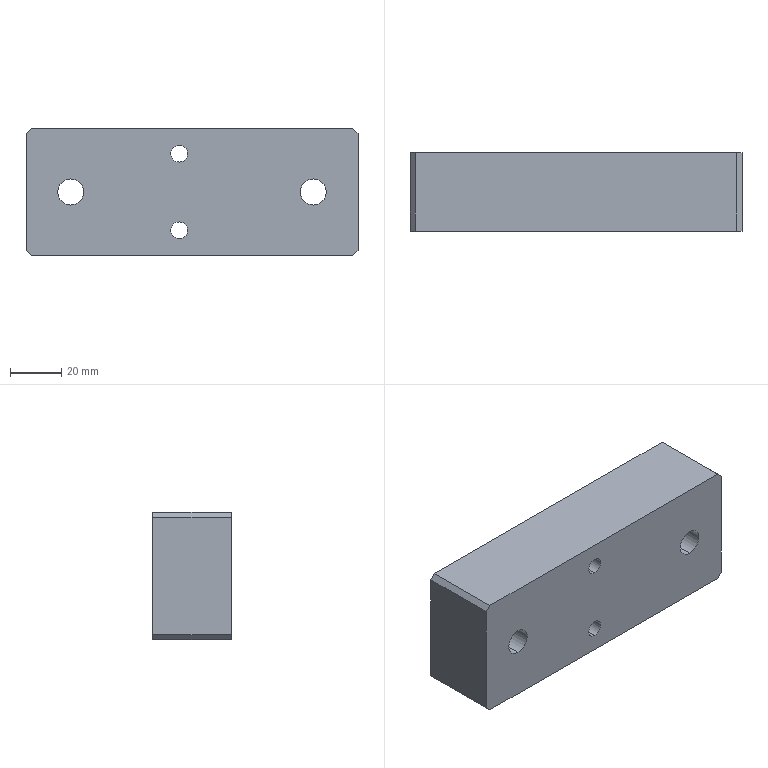Part | SolidWorks | features HoleWzd 2, Chamfer 1, Extrusion 1 | 1 solid | 24 faces | box 130 x 30.7 x 50 mm | volume 191359 mm3 | cylinder 12 | plane 12 | commonest cylinder face diameters 6.6 x4 10.2 x4 11 x4
STEP:
#1=CARTESIAN_POINT('',(-5.,8.55,9.5));
#2=VERTEX_POINT('',#1);
#3=CARTESIAN_POINT('',(-5.,8.55,20.5));
#4=VERTEX_POINT('',#3);
#5=CARTESIAN_POINT('',(-5.,8.55,15.));
#6=DIRECTION('',(0.,1.,0.));
#7=DIRECTION('',(0.,0.,1.));
#8=AXIS2_PLACEMENT_3D('',#5,#6,#7);
#9=CIRCLE('',#8,5.5);
#10=EDGE_CURVE('',#2,#4,#9,.T.);
#11=ORIENTED_EDGE('',*,*,#10,.F.);
#12=CARTESIAN_POINT('',(-5.,15.35,9.5));
#13=VERTEX_POINT('',#12);
#14=CARTESIAN_POINT('',(-5.,15.35,9.5));
#15=DIRECTION('',(0.,1.,0.));
#16=VECTOR('',#15,1000.);
#17=LINE('',#14,#16);
#18=EDGE_CURVE('',#2,#13,#17,.T.);
#19=ORIENTED_EDGE('',*,*,#18,.T.);
#20=CARTESIAN_POINT('',(-5.,15.35,20.5));
#21=VERTEX_POINT('',#20);
#22=CARTESIAN_POINT('',(-5.,15.35,15.));
#23=DIRECTION('',(0.,1.,0.));
#24=DIRECTION('',(0.,0.,1.));
#25=AXIS2_PLACEMENT_3D('',#22,#23,#24);
#26=CIRCLE('',#25,5.5);
#27=EDGE_CURVE('',#13,#21,#26,.T.);
#28=ORIENTED_EDGE('',*,*,#27,.T.);
#29=CARTESIAN_POINT('',(-5.,15.35,20.5));
#30=DIRECTION('',(0.,1.,0.));
#31=VECTOR('',#30,1000.);
#32=LINE('',#29,#31);
#33=EDGE_CURVE('',#4,#21,#32,.T.);
#34=ORIENTED_EDGE('',*,*,#33,.F.);
#35=EDGE_LOOP('',(#11,#19,#28,#34));
#36=FACE_OUTER_BOUND('',#35,.T.);
#37=CARTESIAN_POINT('',(-5.,15.35,15.));
#38=DIRECTION('',(0.,1.,0.));
#39=DIRECTION('',(0.,0.,1.));
#40=AXIS2_PLACEMENT_3D('',#37,#38,#39);
#41=CYLINDRICAL_SURFACE('',#40,5.5);
#42=ADVANCED_FACE('',(#36),#41,.F.);
#43=CARTESIAN_POINT('',(-5.,-15.35,11.7));
#44=VERTEX_POINT('',#43);
#45=CARTESIAN_POINT('',(-5.,-15.35,18.3));
#46=VERTEX_POINT('',#45);
#47=CARTESIAN_POINT('',(-5.,-15.35,15.));
#48=DIRECTION('',(0.,1.,0.));
#49=DIRECTION('',(0.,0.,1.));
#50=AXIS2_PLACEMENT_3D('',#47,#48,#49);
#51=CIRCLE('',#50,3.3);
#52=EDGE_CURVE('',#44,#46,#51,.T.);
#53=ORIENTED_EDGE('',*,*,#52,.F.);
#54=CARTESIAN_POINT('',(-5.,8.55,11.7));
#55=VERTEX_POINT('',#54);
#56=CARTESIAN_POINT('',(-5.,15.35,11.7));
#57=DIRECTION('',(0.,1.,0.));
#58=VECTOR('',#57,1000.);
#59=LINE('',#56,#58);
#60=EDGE_CURVE('',#44,#55,#59,.T.);
#61=ORIENTED_EDGE('',*,*,#60,.T.);
#62=CARTESIAN_POINT('',(-5.,8.55,18.3));
#63=VERTEX_POINT('',#62);
#64=CARTESIAN_POINT('',(-5.,8.55,15.));
#65=DIRECTION('',(0.,1.,0.));
#66=DIRECTION('',(0.,0.,1.));
#67=AXIS2_PLACEMENT_3D('',#64,#65,#66);
#68=CIRCLE('',#67,3.3);
#69=EDGE_CURVE('',#55,#63,#68,.T.);
#70=ORIENTED_EDGE('',*,*,#69,.T.);
#71=CARTESIAN_POINT('',(-5.,15.35,18.3));
#72=DIRECTION('',(0.,1.,0.));
#73=VECTOR('',#72,1000.);
#74=LINE('',#71,#73);
#75=EDGE_CURVE('',#46,#63,#74,.T.);
#76=ORIENTED_EDGE('',*,*,#75,.F.);
#77=EDGE_LOOP('',(#53,#61,#70,#76));
#78=FACE_OUTER_BOUND('',#77,.T.);
#79=CARTESIAN_POINT('',(-5.,15.35,15.));
#80=DIRECTION('',(0.,1.,0.));
#81=DIRECTION('',(0.,0.,1.));
#82=AXIS2_PLACEMENT_3D('',#79,#80,#81);
#83=CYLINDRICAL_SURFACE('',#82,3.3);
#84=ADVANCED_FACE('',(#78),#83,.F.);
#85=CARTESIAN_POINT('',(-5.,8.55,-20.5));
#86=VERTEX_POINT('',#85);
#87=CARTESIAN_POINT('',(-5.,8.55,-9.5));
#88=VERTEX_POINT('',#87);
#89=CARTESIAN_POINT('',(-5.,8.55,-15.));
#90=DIRECTION('',(0.,1.,0.));
#91=DIRECTION('',(0.,0.,1.));
#92=AXIS2_PLACEMENT_3D('',#89,#90,#91);
#93=CIRCLE('',#92,5.5);
#94=EDGE_CURVE('',#86,#88,#93,.T.);
#95=ORIENTED_EDGE('',*,*,#94,.F.);
#96=CARTESIAN_POINT('',(-5.,15.35,-20.5));
#97=VERTEX_POINT('',#96);
#98=CARTESIAN_POINT('',(-5.,15.35,-20.5));
#99=DIRECTION('',(0.,1.,0.));
#100=VECTOR('',#99,1000.);
#101=LINE('',#98,#100);
#102=EDGE_CURVE('',#86,#97,#101,.T.);
#103=ORIENTED_EDGE('',*,*,#102,.T.);
#104=CARTESIAN_POINT('',(-5.,15.35,-9.5));
#105=VERTEX_POINT('',#104);
#106=CARTESIAN_POINT('',(-5.,15.35,-15.));
#107=DIRECTION('',(0.,1.,0.));
#108=DIRECTION('',(0.,0.,1.));
#109=AXIS2_PLACEMENT_3D('',#106,#107,#108);
#110=CIRCLE('',#109,5.5);
#111=EDGE_CURVE('',#97,#105,#110,.T.);
#112=ORIENTED_EDGE('',*,*,#111,.T.);
#113=CARTESIAN_POINT('',(-5.,15.35,-9.5));
#114=DIRECTION('',(0.,1.,0.));
#115=VECTOR('',#114,1000.);
#116=LINE('',#113,#115);
#117=EDGE_CURVE('',#88,#105,#116,.T.);
#118=ORIENTED_EDGE('',*,*,#117,.F.);
#119=EDGE_LOOP('',(#95,#103,#112,#118));
#120=FACE_OUTER_BOUND('',#119,.T.);
#121=CARTESIAN_POINT('',(-5.,15.35,-15.));
#122=DIRECTION('',(0.,1.,0.));
#123=DIRECTION('',(0.,0.,1.));
#124=AXIS2_PLACEMENT_3D('',#121,#122,#123);
#125=CYLINDRICAL_SURFACE('',#124,5.5);
#126=ADVANCED_FACE('',(#120),#125,.F.);
#127=CARTESIAN_POINT('',(-5.,-15.35,-18.3));
#128=VERTEX_POINT('',#127);
#129=CARTESIAN_POINT('',(-5.,-15.35,-11.7));
#130=VERTEX_POINT('',#129);
#131=CARTESIAN_POINT('',(-5.,-15.35,-15.));
#132=DIRECTION('',(0.,1.,0.));
#133=DIRECTION('',(0.,0.,1.));
#134=AXIS2_PLACEMENT_3D('',#131,#132,#133);
#135=CIRCLE('',#134,3.3);
#136=EDGE_CURVE('',#128,#130,#135,.T.);
#137=ORIENTED_EDGE('',*,*,#136,.F.);
#138=CARTESIAN_POINT('',(-5.,8.55,-18.3));
#139=VERTEX_POINT('',#138);
#140=CARTESIAN_POINT('',(-5.,15.35,-18.3));
#141=DIRECTION('',(0.,1.,0.));
#142=VECTOR('',#141,1000.);
#143=LINE('',#140,#142);
#144=EDGE_CURVE('',#128,#139,#143,.T.);
#145=ORIENTED_EDGE('',*,*,#144,.T.);
#146=CARTESIAN_POINT('',(-5.,8.55,-11.7));
#147=VERTEX_POINT('',#146);
#148=CARTESIAN_POINT('',(-5.,8.55,-15.));
#149=DIRECTION('',(0.,1.,0.));
#150=DIRECTION('',(0.,0.,1.));
#151=AXIS2_PLACEMENT_3D('',#148,#149,#150);
#152=CIRCLE('',#151,3.3);
#153=EDGE_CURVE('',#139,#147,#152,.T.);
#154=ORIENTED_EDGE('',*,*,#153,.T.);
#155=CARTESIAN_POINT('',(-5.,15.35,-11.7));
#156=DIRECTION('',(0.,1.,0.));
#157=VECTOR('',#156,1000.);
#158=LINE('',#155,#157);
#159=EDGE_CURVE('',#130,#147,#158,.T.);
#160=ORIENTED_EDGE('',*,*,#159,.F.);
#161=EDGE_LOOP('',(#137,#145,#154,#160));
#162=FACE_OUTER_BOUND('',#161,.T.);
#163=CARTESIAN_POINT('',(-5.,15.35,-15.));
#164=DIRECTION('',(0.,1.,0.));
#165=DIRECTION('',(0.,0.,1.));
#166=AXIS2_PLACEMENT_3D('',#163,#164,#165);
#167=CYLINDRICAL_SURFACE('',#166,3.3);
#168=ADVANCED_FACE('',(#162),#167,.F.);
#169=CARTESIAN_POINT('',(-47.5,-15.35,-5.1));
#170=VERTEX_POINT('',#169);
#171=CARTESIAN_POINT('',(-47.5,-15.35,5.1));
#172=VERTEX_POINT('',#171);
#173=CARTESIAN_POINT('',(-47.5,-15.35,0.));
#174=DIRECTION('',(0.,1.,0.));
#175=DIRECTION('',(0.,0.,1.));
#176=AXIS2_PLACEMENT_3D('',#173,#174,#175);
#177=CIRCLE('',#176,5.1);
#178=EDGE_CURVE('',#170,#172,#177,.T.);
#179=ORIENTED_EDGE('',*,*,#178,.F.);
#180=CARTESIAN_POINT('',(-47.5,15.35,-5.1));
#181=VERTEX_POINT('',#180);
#182=CARTESIAN_POINT('',(-47.5,15.35,-5.1));
#183=DIRECTION('',(0.,1.,0.));
#184=VECTOR('',#183,1000.);
#185=LINE('',#182,#184);
#186=EDGE_CURVE('',#170,#181,#185,.T.);
#187=ORIENTED_EDGE('',*,*,#186,.T.);
#188=CARTESIAN_POINT('',(-47.5,15.35,5.1));
#189=VERTEX_POINT('',#188);
#190=CARTESIAN_POINT('',(-47.5,15.35,0.));
#191=DIRECTION('',(0.,1.,0.));
#192=DIRECTION('',(0.,0.,1.));
#193=AXIS2_PLACEMENT_3D('',#190,#191,#192);
#194=CIRCLE('',#193,5.1);
#195=EDGE_CURVE('',#181,#189,#194,.T.);
#196=ORIENTED_EDGE('',*,*,#195,.T.);
#197=CARTESIAN_POINT('',(-47.5,15.35,5.1));
#198=DIRECTION('',(0.,1.,0.));
#199=VECTOR('',#198,1000.);
#200=LINE('',#197,#199);
#201=EDGE_CURVE('',#172,#189,#200,.T.);
#202=ORIENTED_EDGE('',*,*,#201,.F.);
#203=EDGE_LOOP('',(#179,#187,#196,#202));
#204=FACE_OUTER_BOUND('',#203,.T.);
#205=CARTESIAN_POINT('',(-47.5,15.35,0.));
#206=DIRECTION('',(0.,1.,0.));
#207=DIRECTION('',(0.,0.,1.));
#208=AXIS2_PLACEMENT_3D('',#205,#206,#207);
#209=CYLINDRICAL_SURFACE('',#208,5.1);
#210=ADVANCED_FACE('',(#204),#209,.F.);
#211=CARTESIAN_POINT('',(47.5,-15.35,-5.1));
#212=VERTEX_POINT('',#211);
#213=CARTESIAN_POINT('',(47.5,-15.35,5.1));
#214=VERTEX_POINT('',#213);
#215=CARTESIAN_POINT('',(47.5,-15.35,0.));
#216=DIRECTION('',(0.,1.,0.));
#217=DIRECTION('',(0.,0.,1.));
#218=AXIS2_PLACEMENT_3D('',#215,#216,#217);
#219=CIRCLE('',#218,5.1);
#220=EDGE_CURVE('',#212,#214,#219,.T.);
#221=ORIENTED_EDGE('',*,*,#220,.F.);
#222=CARTESIAN_POINT('',(47.5,15.35,-5.1));
#223=VERTEX_POINT('',#222);
#224=CARTESIAN_POINT('',(47.5,15.35,-5.1));
#225=DIRECTION('',(0.,1.,0.));
#226=VECTOR('',#225,1000.);
#227=LINE('',#224,#226);
#228=EDGE_CURVE('',#212,#223,#227,.T.);
#229=ORIENTED_EDGE('',*,*,#228,.T.);
#230=CARTESIAN_POINT('',(47.5,15.35,5.1));
#231=VERTEX_POINT('',#230);
#232=CARTESIAN_POINT('',(47.5,15.35,0.));
#233=DIRECTION('',(0.,1.,0.));
#234=DIRECTION('',(0.,0.,1.));
#235=AXIS2_PLACEMENT_3D('',#232,#233,#234);
#236=CIRCLE('',#235,5.1);
#237=EDGE_CURVE('',#223,#231,#236,.T.);
#238=ORIENTED_EDGE('',*,*,#237,.T.);
#239=CARTESIAN_POINT('',(47.5,15.35,5.1));
#240=DIRECTION('',(0.,1.,0.));
#241=VECTOR('',#240,1000.);
#242=LINE('',#239,#241);
#243=EDGE_CURVE('',#214,#231,#242,.T.);
#244=ORIENTED_EDGE('',*,*,#243,.F.);
#245=EDGE_LOOP('',(#221,#229,#238,#244));
#246=FACE_OUTER_BOUND('',#245,.T.);
#247=CARTESIAN_POINT('',(47.5,15.35,0.));
#248=DIRECTION('',(0.,1.,0.));
#249=DIRECTION('',(0.,0.,1.));
#250=AXIS2_PLACEMENT_3D('',#247,#248,#249);
#251=CYLINDRICAL_SURFACE('',#250,5.1);
#252=ADVANCED_FACE('',(#246),#251,.F.);
#253=CARTESIAN_POINT('',(65.,-15.35,23.));
#254=VERTEX_POINT('',#253);
#255=CARTESIAN_POINT('',(65.,-15.35,-23.));
#256=VERTEX_POINT('',#255);
#257=CARTESIAN_POINT('',(65.,-15.35,25.));
#258=DIRECTION('',(0.,0.,-1.));
#259=VECTOR('',#258,1000.);
#260=LINE('',#257,#259);
#261=EDGE_CURVE('',#254,#256,#260,.T.);
#262=ORIENTED_EDGE('',*,*,#261,.T.);
#263=CARTESIAN_POINT('',(65.,15.35,-23.));
#264=VERTEX_POINT('',#263);
#265=CARTESIAN_POINT('',(65.,15.35,-23.));
#266=DIRECTION('',(0.,1.,0.));
#267=VECTOR('',#266,1000.);
#268=LINE('',#265,#267);
#269=EDGE_CURVE('',#256,#264,#268,.T.);
#270=ORIENTED_EDGE('',*,*,#269,.T.);
#271=CARTESIAN_POINT('',(65.,15.35,23.));
#272=VERTEX_POINT('',#271);
#273=CARTESIAN_POINT('',(65.,15.35,25.));
#274=DIRECTION('',(0.,0.,-1.));
#275=VECTOR('',#274,1000.);
#276=LINE('',#273,#275);
#277=EDGE_CURVE('',#272,#264,#276,.T.);
#278=ORIENTED_EDGE('',*,*,#277,.F.);
#279=CARTESIAN_POINT('',(65.,15.35,23.));
#280=DIRECTION('',(0.,-1.,0.));
#281=VECTOR('',#280,1000.);
#282=LINE('',#279,#281);
#283=EDGE_CURVE('',#272,#254,#282,.T.);
#284=ORIENTED_EDGE('',*,*,#283,.T.);
#285=EDGE_LOOP('',(#262,#270,#278,#284));
#286=FACE_OUTER_BOUND('',#285,.T.);
#287=CARTESIAN_POINT('',(65.,15.35,25.));
#288=DIRECTION('',(-1.,0.,0.));
#289=DIRECTION('',(0.,0.,1.));
#290=AXIS2_PLACEMENT_3D('',#287,#288,#289);
#291=PLANE('',#290);
#292=ADVANCED_FACE('',(#286),#291,.F.);
#293=CARTESIAN_POINT('',(63.,15.35,-25.));
#294=VERTEX_POINT('',#293);
#295=CARTESIAN_POINT('',(-63.,15.35,-25.));
#296=VERTEX_POINT('',#295);
#297=CARTESIAN_POINT('',(-65.,15.35,-25.));
#298=DIRECTION('',(-1.,0.,0.));
#299=VECTOR('',#298,1000.);
#300=LINE('',#297,#299);
#301=EDGE_CURVE('',#294,#296,#300,.T.);
#302=ORIENTED_EDGE('',*,*,#301,.F.);
#303=CARTESIAN_POINT('',(63.,-15.35,-25.));
#304=VERTEX_POINT('',#303);
#305=CARTESIAN_POINT('',(63.,15.35,-25.));
#306=DIRECTION('',(0.,-1.,0.));
#307=VECTOR('',#306,1000.);
#308=LINE('',#305,#307);
#309=EDGE_CURVE('',#294,#304,#308,.T.);
#310=ORIENTED_EDGE('',*,*,#309,.T.);
#311=CARTESIAN_POINT('',(-63.,-15.35,-25.));
#312=VERTEX_POINT('',#311);
#313=CARTESIAN_POINT('',(-65.,-15.35,-25.));
#314=DIRECTION('',(-1.,0.,0.));
#315=VECTOR('',#314,1000.);
#316=LINE('',#313,#315);
#317=EDGE_CURVE('',#304,#312,#316,.T.);
#318=ORIENTED_EDGE('',*,*,#317,.T.);
#319=CARTESIAN_POINT('',(-63.,15.35,-25.));
#320=DIRECTION('',(0.,1.,0.));
#321=VECTOR('',#320,1000.);
#322=LINE('',#319,#321);
#323=EDGE_CURVE('',#312,#296,#322,.T.);
#324=ORIENTED_EDGE('',*,*,#323,.T.);
#325=EDGE_LOOP('',(#302,#310,#318,#324));
#326=FACE_OUTER_BOUND('',#325,.T.);
#327=CARTESIAN_POINT('',(-65.,15.35,-25.));
#328=DIRECTION('',(0.,0.,1.));
#329=DIRECTION('',(1.,0.,0.));
#330=AXIS2_PLACEMENT_3D('',#327,#328,#329);
#331=PLANE('',#330);
#332=ADVANCED_FACE('',(#326),#331,.F.);
#333=CARTESIAN_POINT('',(-65.,15.35,-23.));
#334=VERTEX_POINT('',#333);
#335=CARTESIAN_POINT('',(-65.,15.35,23.));
#336=VERTEX_POINT('',#335);
#337=CARTESIAN_POINT('',(-65.,15.35,25.));
#338=DIRECTION('',(0.,0.,1.));
#339=VECTOR('',#338,1000.);
#340=LINE('',#337,#339);
#341=EDGE_CURVE('',#334,#336,#340,.T.);
#342=ORIENTED_EDGE('',*,*,#341,.F.);
#343=CARTESIAN_POINT('',(-65.,-15.35,-23.));
#344=VERTEX_POINT('',#343);
#345=CARTESIAN_POINT('',(-65.,15.35,-23.));
#346=DIRECTION('',(0.,-1.,0.));
#347=VECTOR('',#346,1000.);
#348=LINE('',#345,#347);
#349=EDGE_CURVE('',#334,#344,#348,.T.);
#350=ORIENTED_EDGE('',*,*,#349,.T.);
#351=CARTESIAN_POINT('',(-65.,-15.35,23.));
#352=VERTEX_POINT('',#351);
#353=CARTESIAN_POINT('',(-65.,-15.35,25.));
#354=DIRECTION('',(0.,0.,1.));
#355=VECTOR('',#354,1000.);
#356=LINE('',#353,#355);
#357=EDGE_CURVE('',#344,#352,#356,.T.);
#358=ORIENTED_EDGE('',*,*,#357,.T.);
#359=CARTESIAN_POINT('',(-65.,15.35,23.));
#360=DIRECTION('',(0.,1.,0.));
#361=VECTOR('',#360,1000.);
#362=LINE('',#359,#361);
#363=EDGE_CURVE('',#352,#336,#362,.T.);
#364=ORIENTED_EDGE('',*,*,#363,.T.);
#365=EDGE_LOOP('',(#342,#350,#358,#364));
#366=FACE_OUTER_BOUND('',#365,.T.);
#367=CARTESIAN_POINT('',(-65.,15.35,25.));
#368=DIRECTION('',(1.,0.,0.));
#369=DIRECTION('',(0.,0.,-1.));
#370=AXIS2_PLACEMENT_3D('',#367,#368,#369);
#371=PLANE('',#370);
#372=ADVANCED_FACE('',(#366),#371,.F.);
#373=CARTESIAN_POINT('',(-63.,-15.35,25.));
#374=VERTEX_POINT('',#373);
#375=CARTESIAN_POINT('',(63.,-15.35,25.));
#376=VERTEX_POINT('',#375);
#377=CARTESIAN_POINT('',(-65.,-15.35,25.));
#378=DIRECTION('',(1.,0.,0.));
#379=VECTOR('',#378,1000.);
#380=LINE('',#377,#379);
#381=EDGE_CURVE('',#374,#376,#380,.T.);
#382=ORIENTED_EDGE('',*,*,#381,.T.);
#383=CARTESIAN_POINT('',(63.,15.35,25.));
#384=VERTEX_POINT('',#383);
#385=CARTESIAN_POINT('',(63.,15.35,25.));
#386=DIRECTION('',(0.,1.,0.));
#387=VECTOR('',#386,1000.);
#388=LINE('',#385,#387);
#389=EDGE_CURVE('',#376,#384,#388,.T.);
#390=ORIENTED_EDGE('',*,*,#389,.T.);
#391=CARTESIAN_POINT('',(-63.,15.35,25.));
#392=VERTEX_POINT('',#391);
#393=CARTESIAN_POINT('',(-65.,15.35,25.));
#394=DIRECTION('',(1.,0.,0.));
#395=VECTOR('',#394,1000.);
#396=LINE('',#393,#395);
#397=EDGE_CURVE('',#392,#384,#396,.T.);
#398=ORIENTED_EDGE('',*,*,#397,.F.);
#399=CARTESIAN_POINT('',(-63.,15.35,25.));
#400=DIRECTION('',(0.,-1.,0.));
#401=VECTOR('',#400,1000.);
#402=LINE('',#399,#401);
#403=EDGE_CURVE('',#392,#374,#402,.T.);
#404=ORIENTED_EDGE('',*,*,#403,.T.);
#405=EDGE_LOOP('',(#382,#390,#398,#404));
#406=FACE_OUTER_BOUND('',#405,.T.);
#407=CARTESIAN_POINT('',(-65.,15.35,25.));
#408=DIRECTION('',(0.,0.,-1.));
#409=DIRECTION('',(-1.,0.,0.));
#410=AXIS2_PLACEMENT_3D('',#407,#408,#409);
#411=PLANE('',#410);
#412=ADVANCED_FACE('',(#406),#411,.F.);
#413=CARTESIAN_POINT('',(-5.,15.35,15.));
#414=DIRECTION('',(0.,1.,0.));
#415=DIRECTION('',(0.,0.,1.));
#416=AXIS2_PLACEMENT_3D('',#413,#414,#415);
#417=CIRCLE('',#416,5.5);
#418=EDGE_CURVE('',#21,#13,#417,.T.);
#419=ORIENTED_EDGE('',*,*,#418,.F.);
#420=ORIENTED_EDGE('',*,*,#27,.F.);
#421=EDGE_LOOP('',(#419,#420));
#422=FACE_BOUND('',#421,.T.);
#423=CARTESIAN_POINT('',(-5.,15.35,-15.));
#424=DIRECTION('',(0.,1.,0.));
#425=DIRECTION('',(0.,0.,1.));
#426=AXIS2_PLACEMENT_3D('',#423,#424,#425);
#427=CIRCLE('',#426,5.5);
#428=EDGE_CURVE('',#105,#97,#427,.T.);
#429=ORIENTED_EDGE('',*,*,#428,.F.);
#430=ORIENTED_EDGE('',*,*,#111,.F.);
#431=EDGE_LOOP('',(#429,#430));
#432=FACE_BOUND('',#431,.T.);
#433=CARTESIAN_POINT('',(-47.5,15.35,0.));
#434=DIRECTION('',(0.,1.,0.));
#435=DIRECTION('',(0.,0.,1.));
#436=AXIS2_PLACEMENT_3D('',#433,#434,#435);
#437=CIRCLE('',#436,5.1);
#438=EDGE_CURVE('',#189,#181,#437,.T.);
#439=ORIENTED_EDGE('',*,*,#438,.F.);
#440=ORIENTED_EDGE('',*,*,#195,.F.);
#441=EDGE_LOOP('',(#439,#440));
#442=FACE_BOUND('',#441,.T.);
#443=CARTESIAN_POINT('',(47.5,15.35,0.));
#444=DIRECTION('',(0.,1.,0.));
#445=DIRECTION('',(0.,0.,1.));
#446=AXIS2_PLACEMENT_3D('',#443,#444,#445);
#447=CIRCLE('',#446,5.1);
#448=EDGE_CURVE('',#231,#223,#447,.T.);
#449=ORIENTED_EDGE('',*,*,#448,.F.);
#450=ORIENTED_EDGE('',*,*,#237,.F.);
#451=EDGE_LOOP('',(#449,#450));
#452=FACE_BOUND('',#451,.T.);
#453=ORIENTED_EDGE('',*,*,#277,.T.);
#454=CARTESIAN_POINT('',(63.,15.35,-25.));
#455=DIRECTION('',(-0.7071,0.,-0.7071));
#456=VECTOR('',#455,1000.);
#457=LINE('',#454,#456);
#458=EDGE_CURVE('',#264,#294,#457,.T.);
#459=ORIENTED_EDGE('',*,*,#458,.T.);
#460=ORIENTED_EDGE('',*,*,#301,.T.);
#461=CARTESIAN_POINT('',(-65.,15.35,-23.));
#462=DIRECTION('',(-0.7071,0.,0.7071));
#463=VECTOR('',#462,1000.);
#464=LINE('',#461,#463);
#465=EDGE_CURVE('',#296,#334,#464,.T.);
#466=ORIENTED_EDGE('',*,*,#465,.T.);
#467=ORIENTED_EDGE('',*,*,#341,.T.);
#468=CARTESIAN_POINT('',(-63.,15.35,25.));
#469=DIRECTION('',(0.7071,0.,0.7071));
#470=VECTOR('',#469,1000.);
#471=LINE('',#468,#470);
#472=EDGE_CURVE('',#336,#392,#471,.T.);
#473=ORIENTED_EDGE('',*,*,#472,.T.);
#474=ORIENTED_EDGE('',*,*,#397,.T.);
#475=CARTESIAN_POINT('',(65.,15.35,23.));
#476=DIRECTION('',(0.7071,0.,-0.7071));
#477=VECTOR('',#476,1000.);
#478=LINE('',#475,#477);
#479=EDGE_CURVE('',#384,#272,#478,.T.);
#480=ORIENTED_EDGE('',*,*,#479,.T.);
#481=EDGE_LOOP('',(#453,#459,#460,#466,#467,#473,#474,#480));
#482=FACE_OUTER_BOUND('',#481,.T.);
#483=CARTESIAN_POINT('',(0.,15.35,0.));
#484=DIRECTION('',(0.,-1.,0.));
#485=DIRECTION('',(0.,0.,-1.));
#486=AXIS2_PLACEMENT_3D('',#483,#484,#485);
#487=PLANE('',#486);
#488=ADVANCED_FACE('',(#422,#432,#442,#452,#482),#487,.F.);
#489=CARTESIAN_POINT('',(-5.,-15.35,15.));
#490=DIRECTION('',(0.,1.,0.));
#491=DIRECTION('',(0.,0.,1.));
#492=AXIS2_PLACEMENT_3D('',#489,#490,#491);
#493=CIRCLE('',#492,3.3);
#494=EDGE_CURVE('',#46,#44,#493,.T.);
#495=ORIENTED_EDGE('',*,*,#494,.T.);
#496=ORIENTED_EDGE('',*,*,#52,.T.);
#497=EDGE_LOOP('',(#495,#496));
#498=FACE_BOUND('',#497,.T.);
#499=CARTESIAN_POINT('',(-5.,-15.35,-15.));
#500=DIRECTION('',(0.,1.,0.));
#501=DIRECTION('',(0.,0.,1.));
#502=AXIS2_PLACEMENT_3D('',#499,#500,#501);
#503=CIRCLE('',#502,3.3);
#504=EDGE_CURVE('',#130,#128,#503,.T.);
#505=ORIENTED_EDGE('',*,*,#504,.T.);
#506=ORIENTED_EDGE('',*,*,#136,.T.);
#507=EDGE_LOOP('',(#505,#506));
#508=FACE_BOUND('',#507,.T.);
#509=CARTESIAN_POINT('',(-47.5,-15.35,0.));
#510=DIRECTION('',(0.,1.,0.));
#511=DIRECTION('',(0.,0.,1.));
#512=AXIS2_PLACEMENT_3D('',#509,#510,#511);
#513=CIRCLE('',#512,5.1);
#514=EDGE_CURVE('',#172,#170,#513,.T.);
#515=ORIENTED_EDGE('',*,*,#514,.T.);
#516=ORIENTED_EDGE('',*,*,#178,.T.);
#517=EDGE_LOOP('',(#515,#516));
#518=FACE_BOUND('',#517,.T.);
#519=CARTESIAN_POINT('',(47.5,-15.35,0.));
#520=DIRECTION('',(0.,1.,0.));
#521=DIRECTION('',(0.,0.,1.));
#522=AXIS2_PLACEMENT_3D('',#519,#520,#521);
#523=CIRCLE('',#522,5.1);
#524=EDGE_CURVE('',#214,#212,#523,.T.);
#525=ORIENTED_EDGE('',*,*,#524,.T.);
#526=ORIENTED_EDGE('',*,*,#220,.T.);
#527=EDGE_LOOP('',(#525,#526));
#528=FACE_BOUND('',#527,.T.);
#529=ORIENTED_EDGE('',*,*,#317,.F.);
#530=CARTESIAN_POINT('',(44.,-15.35,-44.));
#531=DIRECTION('',(0.7071,0.,0.7071));
#532=VECTOR('',#531,1000.);
#533=LINE('',#530,#532);
#534=EDGE_CURVE('',#304,#256,#533,.T.);
#535=ORIENTED_EDGE('',*,*,#534,.T.);
#536=ORIENTED_EDGE('',*,*,#261,.F.);
#537=CARTESIAN_POINT('',(44.,-15.35,44.));
#538=DIRECTION('',(-0.7071,0.,0.7071));
#539=VECTOR('',#538,1000.);
#540=LINE('',#537,#539);
#541=EDGE_CURVE('',#254,#376,#540,.T.);
#542=ORIENTED_EDGE('',*,*,#541,.T.);
#543=ORIENTED_EDGE('',*,*,#381,.F.);
#544=CARTESIAN_POINT('',(-44.,-15.35,44.));
#545=DIRECTION('',(-0.7071,0.,-0.7071));
#546=VECTOR('',#545,1000.);
#547=LINE('',#544,#546);
#548=EDGE_CURVE('',#374,#352,#547,.T.);
#549=ORIENTED_EDGE('',*,*,#548,.T.);
#550=ORIENTED_EDGE('',*,*,#357,.F.);
#551=CARTESIAN_POINT('',(-44.,-15.35,-44.));
#552=DIRECTION('',(0.7071,0.,-0.7071));
#553=VECTOR('',#552,1000.);
#554=LINE('',#551,#553);
#555=EDGE_CURVE('',#344,#312,#554,.T.);
#556=ORIENTED_EDGE('',*,*,#555,.T.);
#557=EDGE_LOOP('',(#529,#535,#536,#542,#543,#549,#550,#556));
#558=FACE_OUTER_BOUND('',#557,.T.);
#559=CARTESIAN_POINT('',(0.,-15.35,0.));
#560=DIRECTION('',(0.,-1.,0.));
#561=DIRECTION('',(0.,0.,-1.));
#562=AXIS2_PLACEMENT_3D('',#559,#560,#561);
#563=PLANE('',#562);
#564=ADVANCED_FACE('',(#498,#508,#518,#528,#558),#563,.T.);
#565=ORIENTED_EDGE('',*,*,#458,.F.);
#566=ORIENTED_EDGE('',*,*,#269,.F.);
#567=ORIENTED_EDGE('',*,*,#534,.F.);
#568=ORIENTED_EDGE('',*,*,#309,.F.);
#569=EDGE_LOOP('',(#565,#566,#567,#568));
#570=FACE_OUTER_BOUND('',#569,.T.);
#571=CARTESIAN_POINT('',(63.,15.35,-25.));
#572=DIRECTION('',(-0.7071,0.,0.7071));
#573=DIRECTION('',(0.,-1.,0.));
#574=AXIS2_PLACEMENT_3D('',#571,#572,#573);
#575=PLANE('',#574);
#576=ADVANCED_FACE('',(#570),#575,.F.);
#577=ORIENTED_EDGE('',*,*,#479,.F.);
#578=ORIENTED_EDGE('',*,*,#389,.F.);
#579=ORIENTED_EDGE('',*,*,#541,.F.);
#580=ORIENTED_EDGE('',*,*,#283,.F.);
#581=EDGE_LOOP('',(#577,#578,#579,#580));
#582=FACE_OUTER_BOUND('',#581,.T.);
#583=CARTESIAN_POINT('',(65.,15.35,23.));
#584=DIRECTION('',(-0.7071,0.,-0.7071));
#585=DIRECTION('',(0.,-1.,0.));
#586=AXIS2_PLACEMENT_3D('',#583,#584,#585);
#587=PLANE('',#586);
#588=ADVANCED_FACE('',(#582),#587,.F.);
#589=ORIENTED_EDGE('',*,*,#465,.F.);
#590=ORIENTED_EDGE('',*,*,#323,.F.);
#591=ORIENTED_EDGE('',*,*,#555,.F.);
#592=ORIENTED_EDGE('',*,*,#349,.F.);
#593=EDGE_LOOP('',(#589,#590,#591,#592));
#594=FACE_OUTER_BOUND('',#593,.T.);
#595=CARTESIAN_POINT('',(-65.,15.35,-23.));
#596=DIRECTION('',(0.7071,0.,0.7071));
#597=DIRECTION('',(0.,-1.,0.));
#598=AXIS2_PLACEMENT_3D('',#595,#596,#597);
#599=PLANE('',#598);
#600=ADVANCED_FACE('',(#594),#599,.F.);
#601=ORIENTED_EDGE('',*,*,#472,.F.);
#602=ORIENTED_EDGE('',*,*,#363,.F.);
#603=ORIENTED_EDGE('',*,*,#548,.F.);
#604=ORIENTED_EDGE('',*,*,#403,.F.);
#605=EDGE_LOOP('',(#601,#602,#603,#604));
#606=FACE_OUTER_BOUND('',#605,.T.);
#607=CARTESIAN_POINT('',(-63.,15.35,25.));
#608=DIRECTION('',(0.7071,0.,-0.7071));
#609=DIRECTION('',(0.,-1.,0.));
#610=AXIS2_PLACEMENT_3D('',#607,#608,#609);
#611=PLANE('',#610);
#612=ADVANCED_FACE('',(#606),#611,.F.);
#613=ORIENTED_EDGE('',*,*,#228,.F.);
#614=ORIENTED_EDGE('',*,*,#524,.F.);
#615=ORIENTED_EDGE('',*,*,#243,.T.);
#616=ORIENTED_EDGE('',*,*,#448,.T.);
#617=EDGE_LOOP('',(#613,#614,#615,#616));
#618=FACE_OUTER_BOUND('',#617,.T.);
#619=CARTESIAN_POINT('',(47.5,15.35,0.));
#620=DIRECTION('',(0.,1.,0.));
#621=DIRECTION('',(0.,0.,1.));
#622=AXIS2_PLACEMENT_3D('',#619,#620,#621);
#623=CYLINDRICAL_SURFACE('',#622,5.1);
#624=ADVANCED_FACE('',(#618),#623,.F.);
#625=ORIENTED_EDGE('',*,*,#186,.F.);
#626=ORIENTED_EDGE('',*,*,#514,.F.);
#627=ORIENTED_EDGE('',*,*,#201,.T.);
#628=ORIENTED_EDGE('',*,*,#438,.T.);
#629=EDGE_LOOP('',(#625,#626,#627,#628));
#630=FACE_OUTER_BOUND('',#629,.T.);
#631=CARTESIAN_POINT('',(-47.5,15.35,0.));
#632=DIRECTION('',(0.,1.,0.));
#633=DIRECTION('',(0.,0.,1.));
#634=AXIS2_PLACEMENT_3D('',#631,#632,#633);
#635=CYLINDRICAL_SURFACE('',#634,5.1);
#636=ADVANCED_FACE('',(#630),#635,.F.);
#637=ORIENTED_EDGE('',*,*,#144,.F.);
#638=ORIENTED_EDGE('',*,*,#504,.F.);
#639=ORIENTED_EDGE('',*,*,#159,.T.);
#640=CARTESIAN_POINT('',(-5.,8.55,-15.));
#641=DIRECTION('',(0.,1.,0.));
#642=DIRECTION('',(0.,0.,1.));
#643=AXIS2_PLACEMENT_3D('',#640,#641,#642);
#644=CIRCLE('',#643,3.3);
#645=EDGE_CURVE('',#147,#139,#644,.T.);
#646=ORIENTED_EDGE('',*,*,#645,.T.);
#647=EDGE_LOOP('',(#637,#638,#639,#646));
#648=FACE_OUTER_BOUND('',#647,.T.);
#649=CARTESIAN_POINT('',(-5.,15.35,-15.));
#650=DIRECTION('',(0.,1.,0.));
#651=DIRECTION('',(0.,0.,1.));
#652=AXIS2_PLACEMENT_3D('',#649,#650,#651);
#653=CYLINDRICAL_SURFACE('',#652,3.3);
#654=ADVANCED_FACE('',(#648),#653,.F.);
#655=ORIENTED_EDGE('',*,*,#645,.F.);
#656=ORIENTED_EDGE('',*,*,#153,.F.);
#657=EDGE_LOOP('',(#655,#656));
#658=FACE_BOUND('',#657,.T.);
#659=CARTESIAN_POINT('',(-5.,8.55,-15.));
#660=DIRECTION('',(0.,1.,0.));
#661=DIRECTION('',(0.,0.,1.));
#662=AXIS2_PLACEMENT_3D('',#659,#660,#661);
#663=CIRCLE('',#662,5.5);
#664=EDGE_CURVE('',#88,#86,#663,.T.);
#665=ORIENTED_EDGE('',*,*,#664,.T.);
#666=ORIENTED_EDGE('',*,*,#94,.T.);
#667=EDGE_LOOP('',(#665,#666));
#668=FACE_OUTER_BOUND('',#667,.T.);
#669=CARTESIAN_POINT('',(-1.7,8.55,-15.));
#670=DIRECTION('',(0.,-1.,0.));
#671=DIRECTION('',(0.,0.,-1.));
#672=AXIS2_PLACEMENT_3D('',#669,#670,#671);
#673=PLANE('',#672);
#674=ADVANCED_FACE('',(#658,#668),#673,.F.);
#675=ORIENTED_EDGE('',*,*,#102,.F.);
#676=ORIENTED_EDGE('',*,*,#664,.F.);
#677=ORIENTED_EDGE('',*,*,#117,.T.);
#678=ORIENTED_EDGE('',*,*,#428,.T.);
#679=EDGE_LOOP('',(#675,#676,#677,#678));
#680=FACE_OUTER_BOUND('',#679,.T.);
#681=CARTESIAN_POINT('',(-5.,15.35,-15.));
#682=DIRECTION('',(0.,1.,0.));
#683=DIRECTION('',(0.,0.,1.));
#684=AXIS2_PLACEMENT_3D('',#681,#682,#683);
#685=CYLINDRICAL_SURFACE('',#684,5.5);
#686=ADVANCED_FACE('',(#680),#685,.F.);
#687=ORIENTED_EDGE('',*,*,#60,.F.);
#688=ORIENTED_EDGE('',*,*,#494,.F.);
#689=ORIENTED_EDGE('',*,*,#75,.T.);
#690=CARTESIAN_POINT('',(-5.,8.55,15.));
#691=DIRECTION('',(0.,1.,0.));
#692=DIRECTION('',(0.,0.,1.));
#693=AXIS2_PLACEMENT_3D('',#690,#691,#692);
#694=CIRCLE('',#693,3.3);
#695=EDGE_CURVE('',#63,#55,#694,.T.);
#696=ORIENTED_EDGE('',*,*,#695,.T.);
#697=EDGE_LOOP('',(#687,#688,#689,#696));
#698=FACE_OUTER_BOUND('',#697,.T.);
#699=CARTESIAN_POINT('',(-5.,15.35,15.));
#700=DIRECTION('',(0.,1.,0.));
#701=DIRECTION('',(0.,0.,1.));
#702=AXIS2_PLACEMENT_3D('',#699,#700,#701);
#703=CYLINDRICAL_SURFACE('',#702,3.3);
#704=ADVANCED_FACE('',(#698),#703,.F.);
#705=ORIENTED_EDGE('',*,*,#695,.F.);
#706=ORIENTED_EDGE('',*,*,#69,.F.);
#707=EDGE_LOOP('',(#705,#706));
#708=FACE_BOUND('',#707,.T.);
#709=CARTESIAN_POINT('',(-5.,8.55,15.));
#710=DIRECTION('',(0.,1.,0.));
#711=DIRECTION('',(0.,0.,1.));
#712=AXIS2_PLACEMENT_3D('',#709,#710,#711);
#713=CIRCLE('',#712,5.5);
#714=EDGE_CURVE('',#4,#2,#713,.T.);
#715=ORIENTED_EDGE('',*,*,#714,.T.);
#716=ORIENTED_EDGE('',*,*,#10,.T.);
#717=EDGE_LOOP('',(#715,#716));
#718=FACE_OUTER_BOUND('',#717,.T.);
#719=CARTESIAN_POINT('',(-1.7,8.55,15.));
#720=DIRECTION('',(0.,-1.,0.));
#721=DIRECTION('',(0.,0.,-1.));
#722=AXIS2_PLACEMENT_3D('',#719,#720,#721);
#723=PLANE('',#722);
#724=ADVANCED_FACE('',(#708,#718),#723,.F.);
#725=ORIENTED_EDGE('',*,*,#18,.F.);
#726=ORIENTED_EDGE('',*,*,#714,.F.);
#727=ORIENTED_EDGE('',*,*,#33,.T.);
#728=ORIENTED_EDGE('',*,*,#418,.T.);
#729=EDGE_LOOP('',(#725,#726,#727,#728));
#730=FACE_OUTER_BOUND('',#729,.T.);
#731=CARTESIAN_POINT('',(-5.,15.35,15.));
#732=DIRECTION('',(0.,1.,0.));
#733=DIRECTION('',(0.,0.,1.));
#734=AXIS2_PLACEMENT_3D('',#731,#732,#733);
#735=CYLINDRICAL_SURFACE('',#734,5.5);
#736=ADVANCED_FACE('',(#730),#735,.F.);
#737=CLOSED_SHELL('',(#42,#84,#126,#168,#210,#252,#292,#332,#372,#412,#488,#564,#576,#588,#600,#612,#624,#636,#654,#674,#686,#704,#724,#736));
#738=MANIFOLD_SOLID_BREP('',#737);
#739=CARTESIAN_POINT('',(0.,0.,0.));
#740=DIRECTION('',(0.,0.,1.));
#741=DIRECTION('',(1.,0.,0.));
#742=AXIS2_PLACEMENT_3D('',#739,#740,#741);
#743=(LENGTH_UNIT()NAMED_UNIT(*)SI_UNIT(.MILLI.,.METRE.));
#744=UNCERTAINTY_MEASURE_WITH_UNIT(LENGTH_MEASURE(0.00001),#743,'','');
#745=(NAMED_UNIT(*)PLANE_ANGLE_UNIT()SI_UNIT($,.RADIAN.));
#746=(NAMED_UNIT(*)SI_UNIT($,.STERADIAN.)SOLID_ANGLE_UNIT());
#747=(GEOMETRIC_REPRESENTATION_CONTEXT(3)GLOBAL_UNCERTAINTY_ASSIGNED_CONTEXT((#744))GLOBAL_UNIT_ASSIGNED_CONTEXT((#743,#745,#746))REPRESENTATION_CONTEXT('',''));
#748=ADVANCED_BREP_SHAPE_REPRESENTATION('',(#738,#742),#747);